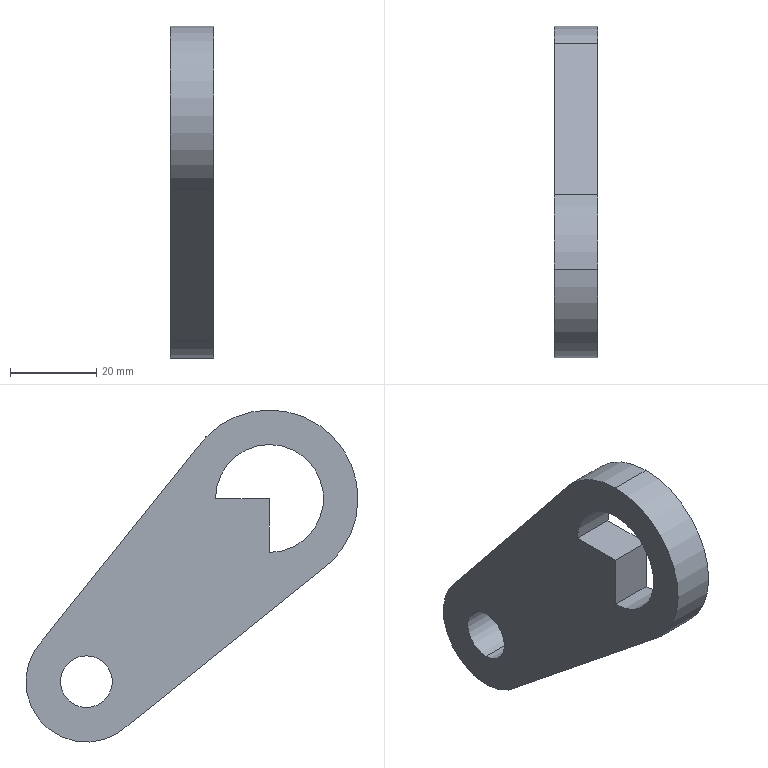Part | SolidWorks | features BaseBody 1 | 1 solid | 13 faces | box 10 x 76.926 x 76.926 mm | volume 25575 mm3 | cylinder 7 | plane 6 | commonest cylinder face diameters 12 x2 25 x2 41 x2 28 x1
STEP:
#1=CARTESIAN_POINT('',(883.833,-3579.973,605.221));
#2=VERTEX_POINT('',#1);
#3=CARTESIAN_POINT('',(883.833,-3591.028,567.458));
#4=VERTEX_POINT('',#3);
#5=CARTESIAN_POINT('',(883.833,-3579.973,584.721));
#6=DIRECTION('',(1.,0.,0.));
#7=DIRECTION('',(0.,0.,1.));
#8=AXIS2_PLACEMENT_3D('',#5,#6,#7);
#9=CIRCLE('',#8,20.5);
#10=EDGE_CURVE('',#2,#4,#9,.T.);
#11=ORIENTED_EDGE('',*,*,#10,.F.);
#12=CARTESIAN_POINT('',(873.833,-3579.973,605.221));
#13=VERTEX_POINT('',#12);
#14=CARTESIAN_POINT('',(883.833,-3579.973,605.221));
#15=DIRECTION('',(-1.,0.,0.));
#16=VECTOR('',#15,1000.);
#17=LINE('',#14,#16);
#18=EDGE_CURVE('',#2,#13,#17,.T.);
#19=ORIENTED_EDGE('',*,*,#18,.T.);
#20=CARTESIAN_POINT('',(873.833,-3591.028,567.458));
#21=VERTEX_POINT('',#20);
#22=CARTESIAN_POINT('',(873.833,-3579.973,584.721));
#23=DIRECTION('',(1.,0.,0.));
#24=DIRECTION('',(0.,0.,1.));
#25=AXIS2_PLACEMENT_3D('',#22,#23,#24);
#26=CIRCLE('',#25,20.5);
#27=EDGE_CURVE('',#13,#21,#26,.T.);
#28=ORIENTED_EDGE('',*,*,#27,.T.);
#29=CARTESIAN_POINT('',(883.833,-3591.028,567.458));
#30=DIRECTION('',(1.,0.,0.));
#31=VECTOR('',#30,1000.);
#32=LINE('',#29,#31);
#33=EDGE_CURVE('',#21,#4,#32,.T.);
#34=ORIENTED_EDGE('',*,*,#33,.T.);
#35=EDGE_LOOP('',(#11,#19,#28,#34));
#36=FACE_OUTER_BOUND('',#35,.T.);
#37=CARTESIAN_POINT('',(883.833,-3579.973,584.721));
#38=DIRECTION('',(-1.,0.,0.));
#39=DIRECTION('',(0.,0.,1.));
#40=AXIS2_PLACEMENT_3D('',#37,#38,#39);
#41=CYLINDRICAL_SURFACE('',#40,20.5);
#42=ADVANCED_FACE('',(#36),#41,.T.);
#43=CARTESIAN_POINT('',(883.833,-3537.547,536.295));
#44=VERTEX_POINT('',#43);
#45=CARTESIAN_POINT('',(883.833,-3537.547,548.295));
#46=VERTEX_POINT('',#45);
#47=CARTESIAN_POINT('',(883.833,-3537.547,542.295));
#48=DIRECTION('',(-1.,0.,0.));
#49=DIRECTION('',(0.,0.,1.));
#50=AXIS2_PLACEMENT_3D('',#47,#48,#49);
#51=CIRCLE('',#50,6.);
#52=EDGE_CURVE('',#44,#46,#51,.T.);
#53=ORIENTED_EDGE('',*,*,#52,.F.);
#54=CARTESIAN_POINT('',(873.833,-3537.547,536.295));
#55=VERTEX_POINT('',#54);
#56=CARTESIAN_POINT('',(883.833,-3537.547,536.295));
#57=DIRECTION('',(-1.,0.,0.));
#58=VECTOR('',#57,1000.);
#59=LINE('',#56,#58);
#60=EDGE_CURVE('',#44,#55,#59,.T.);
#61=ORIENTED_EDGE('',*,*,#60,.T.);
#62=CARTESIAN_POINT('',(873.833,-3537.547,548.295));
#63=VERTEX_POINT('',#62);
#64=CARTESIAN_POINT('',(873.833,-3537.547,542.295));
#65=DIRECTION('',(-1.,0.,0.));
#66=DIRECTION('',(0.,0.,1.));
#67=AXIS2_PLACEMENT_3D('',#64,#65,#66);
#68=CIRCLE('',#67,6.);
#69=EDGE_CURVE('',#55,#63,#68,.T.);
#70=ORIENTED_EDGE('',*,*,#69,.T.);
#71=CARTESIAN_POINT('',(883.833,-3537.547,548.295));
#72=DIRECTION('',(-1.,0.,0.));
#73=VECTOR('',#72,1000.);
#74=LINE('',#71,#73);
#75=EDGE_CURVE('',#46,#63,#74,.T.);
#76=ORIENTED_EDGE('',*,*,#75,.F.);
#77=EDGE_LOOP('',(#53,#61,#70,#76));
#78=FACE_OUTER_BOUND('',#77,.T.);
#79=CARTESIAN_POINT('',(883.833,-3537.547,542.295));
#80=DIRECTION('',(-1.,0.,0.));
#81=DIRECTION('',(0.,0.,1.));
#82=AXIS2_PLACEMENT_3D('',#79,#80,#81);
#83=CYLINDRICAL_SURFACE('',#82,6.);
#84=ADVANCED_FACE('',(#78),#83,.F.);
#85=CARTESIAN_POINT('',(883.833,-3579.973,597.221));
#86=VERTEX_POINT('',#85);
#87=CARTESIAN_POINT('',(883.833,-3567.473,584.721));
#88=VERTEX_POINT('',#87);
#89=CARTESIAN_POINT('',(883.833,-3579.973,584.721));
#90=DIRECTION('',(-1.,0.,0.));
#91=DIRECTION('',(0.,0.,1.));
#92=AXIS2_PLACEMENT_3D('',#89,#90,#91);
#93=CIRCLE('',#92,12.5);
#94=EDGE_CURVE('',#86,#88,#93,.T.);
#95=ORIENTED_EDGE('',*,*,#94,.F.);
#96=CARTESIAN_POINT('',(873.833,-3579.973,597.221));
#97=VERTEX_POINT('',#96);
#98=CARTESIAN_POINT('',(883.833,-3579.973,597.221));
#99=DIRECTION('',(-1.,0.,0.));
#100=VECTOR('',#99,1000.);
#101=LINE('',#98,#100);
#102=EDGE_CURVE('',#86,#97,#101,.T.);
#103=ORIENTED_EDGE('',*,*,#102,.T.);
#104=CARTESIAN_POINT('',(873.833,-3567.473,584.721));
#105=VERTEX_POINT('',#104);
#106=CARTESIAN_POINT('',(873.833,-3579.973,584.721));
#107=DIRECTION('',(-1.,0.,0.));
#108=DIRECTION('',(0.,0.,1.));
#109=AXIS2_PLACEMENT_3D('',#106,#107,#108);
#110=CIRCLE('',#109,12.5);
#111=EDGE_CURVE('',#97,#105,#110,.T.);
#112=ORIENTED_EDGE('',*,*,#111,.T.);
#113=CARTESIAN_POINT('',(883.833,-3567.473,584.721));
#114=DIRECTION('',(1.,0.,0.));
#115=VECTOR('',#114,1000.);
#116=LINE('',#113,#115);
#117=EDGE_CURVE('',#105,#88,#116,.T.);
#118=ORIENTED_EDGE('',*,*,#117,.T.);
#119=EDGE_LOOP('',(#95,#103,#112,#118));
#120=FACE_OUTER_BOUND('',#119,.T.);
#121=CARTESIAN_POINT('',(883.833,-3579.973,584.721));
#122=DIRECTION('',(-1.,0.,0.));
#123=DIRECTION('',(0.,0.,1.));
#124=AXIS2_PLACEMENT_3D('',#121,#122,#123);
#125=CYLINDRICAL_SURFACE('',#124,12.5);
#126=ADVANCED_FACE('',(#120),#125,.F.);
#127=CARTESIAN_POINT('',(883.833,-3527.647,552.195));
#128=VERTEX_POINT('',#127);
#129=CARTESIAN_POINT('',(883.833,-3562.709,595.777));
#130=VERTEX_POINT('',#129);
#131=CARTESIAN_POINT('',(883.833,-3527.647,552.195));
#132=DIRECTION('',(0.,-0.6268,0.7792));
#133=VECTOR('',#132,1000.);
#134=LINE('',#131,#133);
#135=EDGE_CURVE('',#128,#130,#134,.T.);
#136=ORIENTED_EDGE('',*,*,#135,.T.);
#137=CARTESIAN_POINT('',(883.833,-3579.973,584.721));
#138=DIRECTION('',(1.,0.,0.));
#139=DIRECTION('',(0.,0.,1.));
#140=AXIS2_PLACEMENT_3D('',#137,#138,#139);
#141=CIRCLE('',#140,20.5);
#142=EDGE_CURVE('',#130,#2,#141,.T.);
#143=ORIENTED_EDGE('',*,*,#142,.T.);
#144=ORIENTED_EDGE('',*,*,#10,.T.);
#145=CARTESIAN_POINT('',(883.833,-3547.446,532.396));
#146=VERTEX_POINT('',#145);
#147=CARTESIAN_POINT('',(883.833,-3591.028,567.458));
#148=DIRECTION('',(0.,0.7792,-0.6268));
#149=VECTOR('',#148,1000.);
#150=LINE('',#147,#149);
#151=EDGE_CURVE('',#4,#146,#150,.T.);
#152=ORIENTED_EDGE('',*,*,#151,.T.);
#153=CARTESIAN_POINT('',(883.833,-3537.547,542.295));
#154=DIRECTION('',(1.,0.,0.));
#155=DIRECTION('',(0.,0.,1.));
#156=AXIS2_PLACEMENT_3D('',#153,#154,#155);
#157=CIRCLE('',#156,14.);
#158=EDGE_CURVE('',#146,#128,#157,.T.);
#159=ORIENTED_EDGE('',*,*,#158,.T.);
#160=EDGE_LOOP('',(#136,#143,#144,#152,#159));
#161=FACE_OUTER_BOUND('',#160,.T.);
#162=CARTESIAN_POINT('',(883.833,-3537.547,542.295));
#163=DIRECTION('',(-1.,0.,0.));
#164=DIRECTION('',(0.,0.,1.));
#165=AXIS2_PLACEMENT_3D('',#162,#163,#164);
#166=CIRCLE('',#165,6.);
#167=EDGE_CURVE('',#46,#44,#166,.T.);
#168=ORIENTED_EDGE('',*,*,#167,.T.);
#169=ORIENTED_EDGE('',*,*,#52,.T.);
#170=EDGE_LOOP('',(#168,#169));
#171=FACE_BOUND('',#170,.T.);
#172=CARTESIAN_POINT('',(883.833,-3579.973,584.721));
#173=VERTEX_POINT('',#172);
#174=CARTESIAN_POINT('',(883.833,-3579.973,572.221));
#175=VERTEX_POINT('',#174);
#176=CARTESIAN_POINT('',(883.833,-3579.973,566.558));
#177=DIRECTION('',(0.,0.,-1.));
#178=VECTOR('',#177,1000.);
#179=LINE('',#176,#178);
#180=EDGE_CURVE('',#173,#175,#179,.T.);
#181=ORIENTED_EDGE('',*,*,#180,.T.);
#182=CARTESIAN_POINT('',(883.833,-3579.973,584.721));
#183=DIRECTION('',(-1.,0.,0.));
#184=DIRECTION('',(0.,0.,1.));
#185=AXIS2_PLACEMENT_3D('',#182,#183,#184);
#186=CIRCLE('',#185,12.5);
#187=EDGE_CURVE('',#175,#86,#186,.T.);
#188=ORIENTED_EDGE('',*,*,#187,.T.);
#189=ORIENTED_EDGE('',*,*,#94,.T.);
#190=CARTESIAN_POINT('',(883.833,-3561.81,584.721));
#191=DIRECTION('',(0.,-1.,0.));
#192=VECTOR('',#191,1000.);
#193=LINE('',#190,#192);
#194=EDGE_CURVE('',#88,#173,#193,.T.);
#195=ORIENTED_EDGE('',*,*,#194,.T.);
#196=EDGE_LOOP('',(#181,#188,#189,#195));
#197=FACE_BOUND('',#196,.T.);
#198=CARTESIAN_POINT('',(883.833,-3561.81,566.558));
#199=DIRECTION('',(1.,0.,0.));
#200=DIRECTION('',(0.,0.,-1.));
#201=AXIS2_PLACEMENT_3D('',#198,#199,#200);
#202=PLANE('',#201);
#203=ADVANCED_FACE('',(#161,#171,#197),#202,.T.);
#204=ORIENTED_EDGE('',*,*,#18,.F.);
#205=ORIENTED_EDGE('',*,*,#142,.F.);
#206=CARTESIAN_POINT('',(873.833,-3562.709,595.777));
#207=VERTEX_POINT('',#206);
#208=CARTESIAN_POINT('',(883.833,-3562.709,595.777));
#209=DIRECTION('',(-1.,0.,0.));
#210=VECTOR('',#209,1000.);
#211=LINE('',#208,#210);
#212=EDGE_CURVE('',#130,#207,#211,.T.);
#213=ORIENTED_EDGE('',*,*,#212,.T.);
#214=CARTESIAN_POINT('',(873.833,-3579.973,584.721));
#215=DIRECTION('',(1.,0.,0.));
#216=DIRECTION('',(0.,0.,1.));
#217=AXIS2_PLACEMENT_3D('',#214,#215,#216);
#218=CIRCLE('',#217,20.5);
#219=EDGE_CURVE('',#207,#13,#218,.T.);
#220=ORIENTED_EDGE('',*,*,#219,.T.);
#221=EDGE_LOOP('',(#204,#205,#213,#220));
#222=FACE_OUTER_BOUND('',#221,.T.);
#223=CARTESIAN_POINT('',(883.833,-3579.973,584.721));
#224=DIRECTION('',(-1.,0.,0.));
#225=DIRECTION('',(0.,0.,1.));
#226=AXIS2_PLACEMENT_3D('',#223,#224,#225);
#227=CYLINDRICAL_SURFACE('',#226,20.5);
#228=ADVANCED_FACE('',(#222),#227,.T.);
#229=ORIENTED_EDGE('',*,*,#135,.F.);
#230=CARTESIAN_POINT('',(873.833,-3527.647,552.195));
#231=VERTEX_POINT('',#230);
#232=CARTESIAN_POINT('',(883.833,-3527.647,552.195));
#233=DIRECTION('',(-1.,0.,0.));
#234=VECTOR('',#233,1000.);
#235=LINE('',#232,#234);
#236=EDGE_CURVE('',#128,#231,#235,.T.);
#237=ORIENTED_EDGE('',*,*,#236,.T.);
#238=CARTESIAN_POINT('',(873.833,-3527.647,552.195));
#239=DIRECTION('',(0.,-0.6268,0.7792));
#240=VECTOR('',#239,1000.);
#241=LINE('',#238,#240);
#242=EDGE_CURVE('',#231,#207,#241,.T.);
#243=ORIENTED_EDGE('',*,*,#242,.T.);
#244=ORIENTED_EDGE('',*,*,#212,.F.);
#245=EDGE_LOOP('',(#229,#237,#243,#244));
#246=FACE_OUTER_BOUND('',#245,.T.);
#247=CARTESIAN_POINT('',(883.833,-3527.647,552.195));
#248=DIRECTION('',(0.,0.7792,0.6268));
#249=DIRECTION('',(0.,-0.6268,0.7792));
#250=AXIS2_PLACEMENT_3D('',#247,#248,#249);
#251=PLANE('',#250);
#252=ADVANCED_FACE('',(#246),#251,.T.);
#253=ORIENTED_EDGE('',*,*,#158,.F.);
#254=CARTESIAN_POINT('',(873.833,-3547.446,532.396));
#255=VERTEX_POINT('',#254);
#256=CARTESIAN_POINT('',(883.833,-3547.446,532.396));
#257=DIRECTION('',(-1.,0.,0.));
#258=VECTOR('',#257,1000.);
#259=LINE('',#256,#258);
#260=EDGE_CURVE('',#146,#255,#259,.T.);
#261=ORIENTED_EDGE('',*,*,#260,.T.);
#262=CARTESIAN_POINT('',(873.833,-3537.547,542.295));
#263=DIRECTION('',(1.,0.,0.));
#264=DIRECTION('',(0.,0.,1.));
#265=AXIS2_PLACEMENT_3D('',#262,#263,#264);
#266=CIRCLE('',#265,14.);
#267=EDGE_CURVE('',#255,#231,#266,.T.);
#268=ORIENTED_EDGE('',*,*,#267,.T.);
#269=ORIENTED_EDGE('',*,*,#236,.F.);
#270=EDGE_LOOP('',(#253,#261,#268,#269));
#271=FACE_OUTER_BOUND('',#270,.T.);
#272=CARTESIAN_POINT('',(883.833,-3537.547,542.295));
#273=DIRECTION('',(-1.,0.,0.));
#274=DIRECTION('',(0.,0.,1.));
#275=AXIS2_PLACEMENT_3D('',#272,#273,#274);
#276=CYLINDRICAL_SURFACE('',#275,14.);
#277=ADVANCED_FACE('',(#271),#276,.T.);
#278=ORIENTED_EDGE('',*,*,#151,.F.);
#279=ORIENTED_EDGE('',*,*,#33,.F.);
#280=CARTESIAN_POINT('',(873.833,-3591.028,567.458));
#281=DIRECTION('',(0.,0.7792,-0.6268));
#282=VECTOR('',#281,1000.);
#283=LINE('',#280,#282);
#284=EDGE_CURVE('',#21,#255,#283,.T.);
#285=ORIENTED_EDGE('',*,*,#284,.T.);
#286=ORIENTED_EDGE('',*,*,#260,.F.);
#287=EDGE_LOOP('',(#278,#279,#285,#286));
#288=FACE_OUTER_BOUND('',#287,.T.);
#289=CARTESIAN_POINT('',(883.833,-3591.028,567.458));
#290=DIRECTION('',(0.,-0.6268,-0.7792));
#291=DIRECTION('',(0.,0.7792,-0.6268));
#292=AXIS2_PLACEMENT_3D('',#289,#290,#291);
#293=PLANE('',#292);
#294=ADVANCED_FACE('',(#288),#293,.T.);
#295=ORIENTED_EDGE('',*,*,#60,.F.);
#296=ORIENTED_EDGE('',*,*,#167,.F.);
#297=ORIENTED_EDGE('',*,*,#75,.T.);
#298=CARTESIAN_POINT('',(873.833,-3537.547,542.295));
#299=DIRECTION('',(-1.,0.,0.));
#300=DIRECTION('',(0.,0.,1.));
#301=AXIS2_PLACEMENT_3D('',#298,#299,#300);
#302=CIRCLE('',#301,6.);
#303=EDGE_CURVE('',#63,#55,#302,.T.);
#304=ORIENTED_EDGE('',*,*,#303,.T.);
#305=EDGE_LOOP('',(#295,#296,#297,#304));
#306=FACE_OUTER_BOUND('',#305,.T.);
#307=CARTESIAN_POINT('',(883.833,-3537.547,542.295));
#308=DIRECTION('',(-1.,0.,0.));
#309=DIRECTION('',(0.,0.,1.));
#310=AXIS2_PLACEMENT_3D('',#307,#308,#309);
#311=CYLINDRICAL_SURFACE('',#310,6.);
#312=ADVANCED_FACE('',(#306),#311,.F.);
#313=ORIENTED_EDGE('',*,*,#102,.F.);
#314=ORIENTED_EDGE('',*,*,#187,.F.);
#315=CARTESIAN_POINT('',(873.833,-3579.973,572.221));
#316=VERTEX_POINT('',#315);
#317=CARTESIAN_POINT('',(883.833,-3579.973,572.221));
#318=DIRECTION('',(-1.,0.,0.));
#319=VECTOR('',#318,1000.);
#320=LINE('',#317,#319);
#321=EDGE_CURVE('',#175,#316,#320,.T.);
#322=ORIENTED_EDGE('',*,*,#321,.T.);
#323=CARTESIAN_POINT('',(873.833,-3579.973,584.721));
#324=DIRECTION('',(-1.,0.,0.));
#325=DIRECTION('',(0.,0.,1.));
#326=AXIS2_PLACEMENT_3D('',#323,#324,#325);
#327=CIRCLE('',#326,12.5);
#328=EDGE_CURVE('',#316,#97,#327,.T.);
#329=ORIENTED_EDGE('',*,*,#328,.T.);
#330=EDGE_LOOP('',(#313,#314,#322,#329));
#331=FACE_OUTER_BOUND('',#330,.T.);
#332=CARTESIAN_POINT('',(883.833,-3579.973,584.721));
#333=DIRECTION('',(-1.,0.,0.));
#334=DIRECTION('',(0.,0.,1.));
#335=AXIS2_PLACEMENT_3D('',#332,#333,#334);
#336=CYLINDRICAL_SURFACE('',#335,12.5);
#337=ADVANCED_FACE('',(#331),#336,.F.);
#338=ORIENTED_EDGE('',*,*,#180,.F.);
#339=CARTESIAN_POINT('',(873.833,-3579.973,584.721));
#340=VERTEX_POINT('',#339);
#341=CARTESIAN_POINT('',(883.833,-3579.973,584.721));
#342=DIRECTION('',(-1.,0.,0.));
#343=VECTOR('',#342,1000.);
#344=LINE('',#341,#343);
#345=EDGE_CURVE('',#173,#340,#344,.T.);
#346=ORIENTED_EDGE('',*,*,#345,.T.);
#347=CARTESIAN_POINT('',(873.833,-3579.973,584.721));
#348=DIRECTION('',(0.,0.,-1.));
#349=VECTOR('',#348,1000.);
#350=LINE('',#347,#349);
#351=EDGE_CURVE('',#340,#316,#350,.T.);
#352=ORIENTED_EDGE('',*,*,#351,.T.);
#353=ORIENTED_EDGE('',*,*,#321,.F.);
#354=EDGE_LOOP('',(#338,#346,#352,#353));
#355=FACE_OUTER_BOUND('',#354,.T.);
#356=CARTESIAN_POINT('',(883.833,-3579.973,584.721));
#357=DIRECTION('',(0.,-1.,0.));
#358=DIRECTION('',(0.,0.,-1.));
#359=AXIS2_PLACEMENT_3D('',#356,#357,#358);
#360=PLANE('',#359);
#361=ADVANCED_FACE('',(#355),#360,.T.);
#362=ORIENTED_EDGE('',*,*,#194,.F.);
#363=ORIENTED_EDGE('',*,*,#117,.F.);
#364=CARTESIAN_POINT('',(873.833,-3567.473,584.721));
#365=DIRECTION('',(0.,-1.,0.));
#366=VECTOR('',#365,1000.);
#367=LINE('',#364,#366);
#368=EDGE_CURVE('',#105,#340,#367,.T.);
#369=ORIENTED_EDGE('',*,*,#368,.T.);
#370=ORIENTED_EDGE('',*,*,#345,.F.);
#371=EDGE_LOOP('',(#362,#363,#369,#370));
#372=FACE_OUTER_BOUND('',#371,.T.);
#373=CARTESIAN_POINT('',(883.833,-3567.473,584.721));
#374=DIRECTION('',(0.,0.,1.));
#375=DIRECTION('',(0.,-1.,0.));
#376=AXIS2_PLACEMENT_3D('',#373,#374,#375);
#377=PLANE('',#376);
#378=ADVANCED_FACE('',(#372),#377,.T.);
#379=ORIENTED_EDGE('',*,*,#284,.F.);
#380=ORIENTED_EDGE('',*,*,#27,.F.);
#381=ORIENTED_EDGE('',*,*,#219,.F.);
#382=ORIENTED_EDGE('',*,*,#242,.F.);
#383=ORIENTED_EDGE('',*,*,#267,.F.);
#384=EDGE_LOOP('',(#379,#380,#381,#382,#383));
#385=FACE_OUTER_BOUND('',#384,.T.);
#386=ORIENTED_EDGE('',*,*,#303,.F.);
#387=ORIENTED_EDGE('',*,*,#69,.F.);
#388=EDGE_LOOP('',(#386,#387));
#389=FACE_BOUND('',#388,.T.);
#390=ORIENTED_EDGE('',*,*,#368,.F.);
#391=ORIENTED_EDGE('',*,*,#111,.F.);
#392=ORIENTED_EDGE('',*,*,#328,.F.);
#393=ORIENTED_EDGE('',*,*,#351,.F.);
#394=EDGE_LOOP('',(#390,#391,#392,#393));
#395=FACE_BOUND('',#394,.T.);
#396=CARTESIAN_POINT('',(873.833,-3561.81,566.558));
#397=DIRECTION('',(1.,0.,0.));
#398=DIRECTION('',(0.,0.,-1.));
#399=AXIS2_PLACEMENT_3D('',#396,#397,#398);
#400=PLANE('',#399);
#401=ADVANCED_FACE('',(#385,#389,#395),#400,.F.);
#402=CLOSED_SHELL('',(#42,#84,#126,#203,#228,#252,#277,#294,#312,#337,#361,#378,#401));
#403=MANIFOLD_SOLID_BREP('',#402);
#404=CARTESIAN_POINT('',(0.,0.,0.));
#405=DIRECTION('',(0.,0.,1.));
#406=DIRECTION('',(1.,0.,0.));
#407=AXIS2_PLACEMENT_3D('',#404,#405,#406);
#408=(LENGTH_UNIT()NAMED_UNIT(*)SI_UNIT(.MILLI.,.METRE.));
#409=UNCERTAINTY_MEASURE_WITH_UNIT(LENGTH_MEASURE(0.00001),#408,'','');
#410=(NAMED_UNIT(*)PLANE_ANGLE_UNIT()SI_UNIT($,.RADIAN.));
#411=(NAMED_UNIT(*)SI_UNIT($,.STERADIAN.)SOLID_ANGLE_UNIT());
#412=(GEOMETRIC_REPRESENTATION_CONTEXT(3)GLOBAL_UNCERTAINTY_ASSIGNED_CONTEXT((#409))GLOBAL_UNIT_ASSIGNED_CONTEXT((#408,#410,#411))REPRESENTATION_CONTEXT('',''));
#413=ADVANCED_BREP_SHAPE_REPRESENTATION('',(#403,#407),#412);